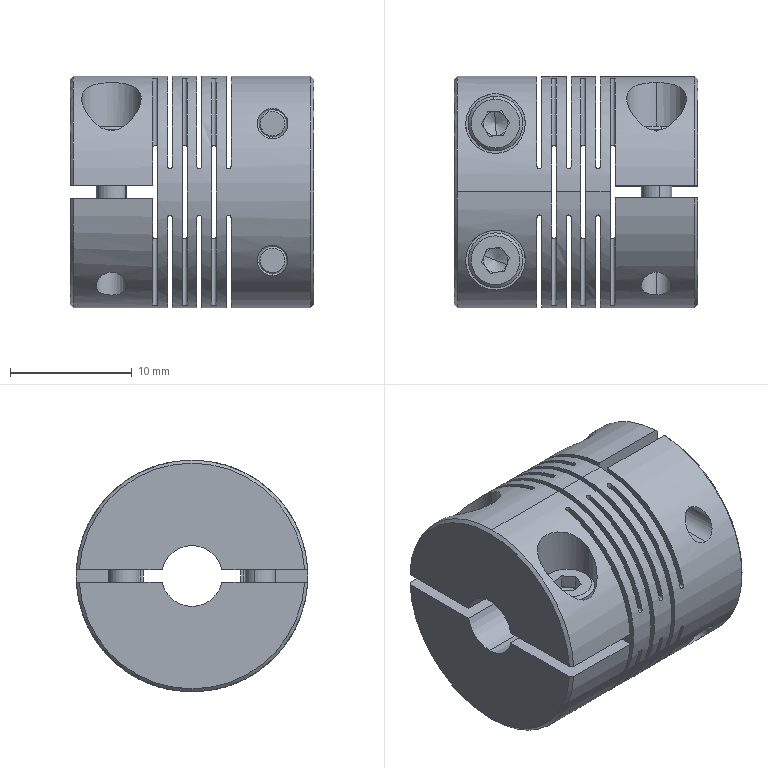Part | SolidWorks | features AEMSimFeature 1 | 5 solids | 232 faces | box 20 x 19 x 19 mm | volume 4000 mm3 | plane 100 | cylinder 87 | cone 45 | commonest cylinder face diameters 0.4 x30 2.5 x24 2.013 x8 4.5 x8 4.9 x8 5 x3